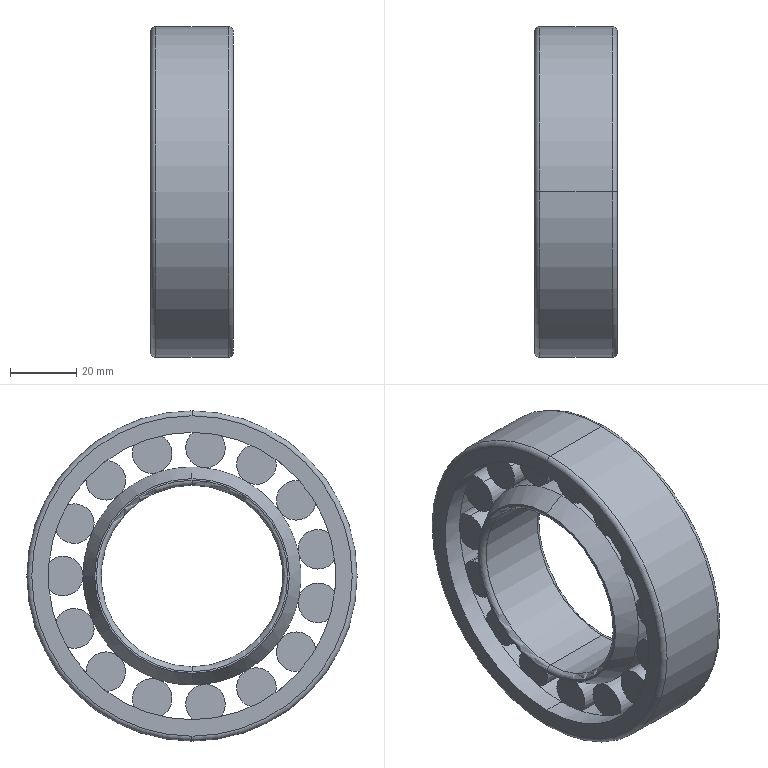Part | SolidWorks | features Revolution 3, CirPattern 1 | 1 solid | 161 faces | box 25 x 100 x 100 mm | volume 86122 mm3 | cylinder 85 | plane 64 | torus 8 | cone 4 | commonest cylinder face diameters 12 x45 66 x16 90 x16 87 x4 55 x2 100 x2